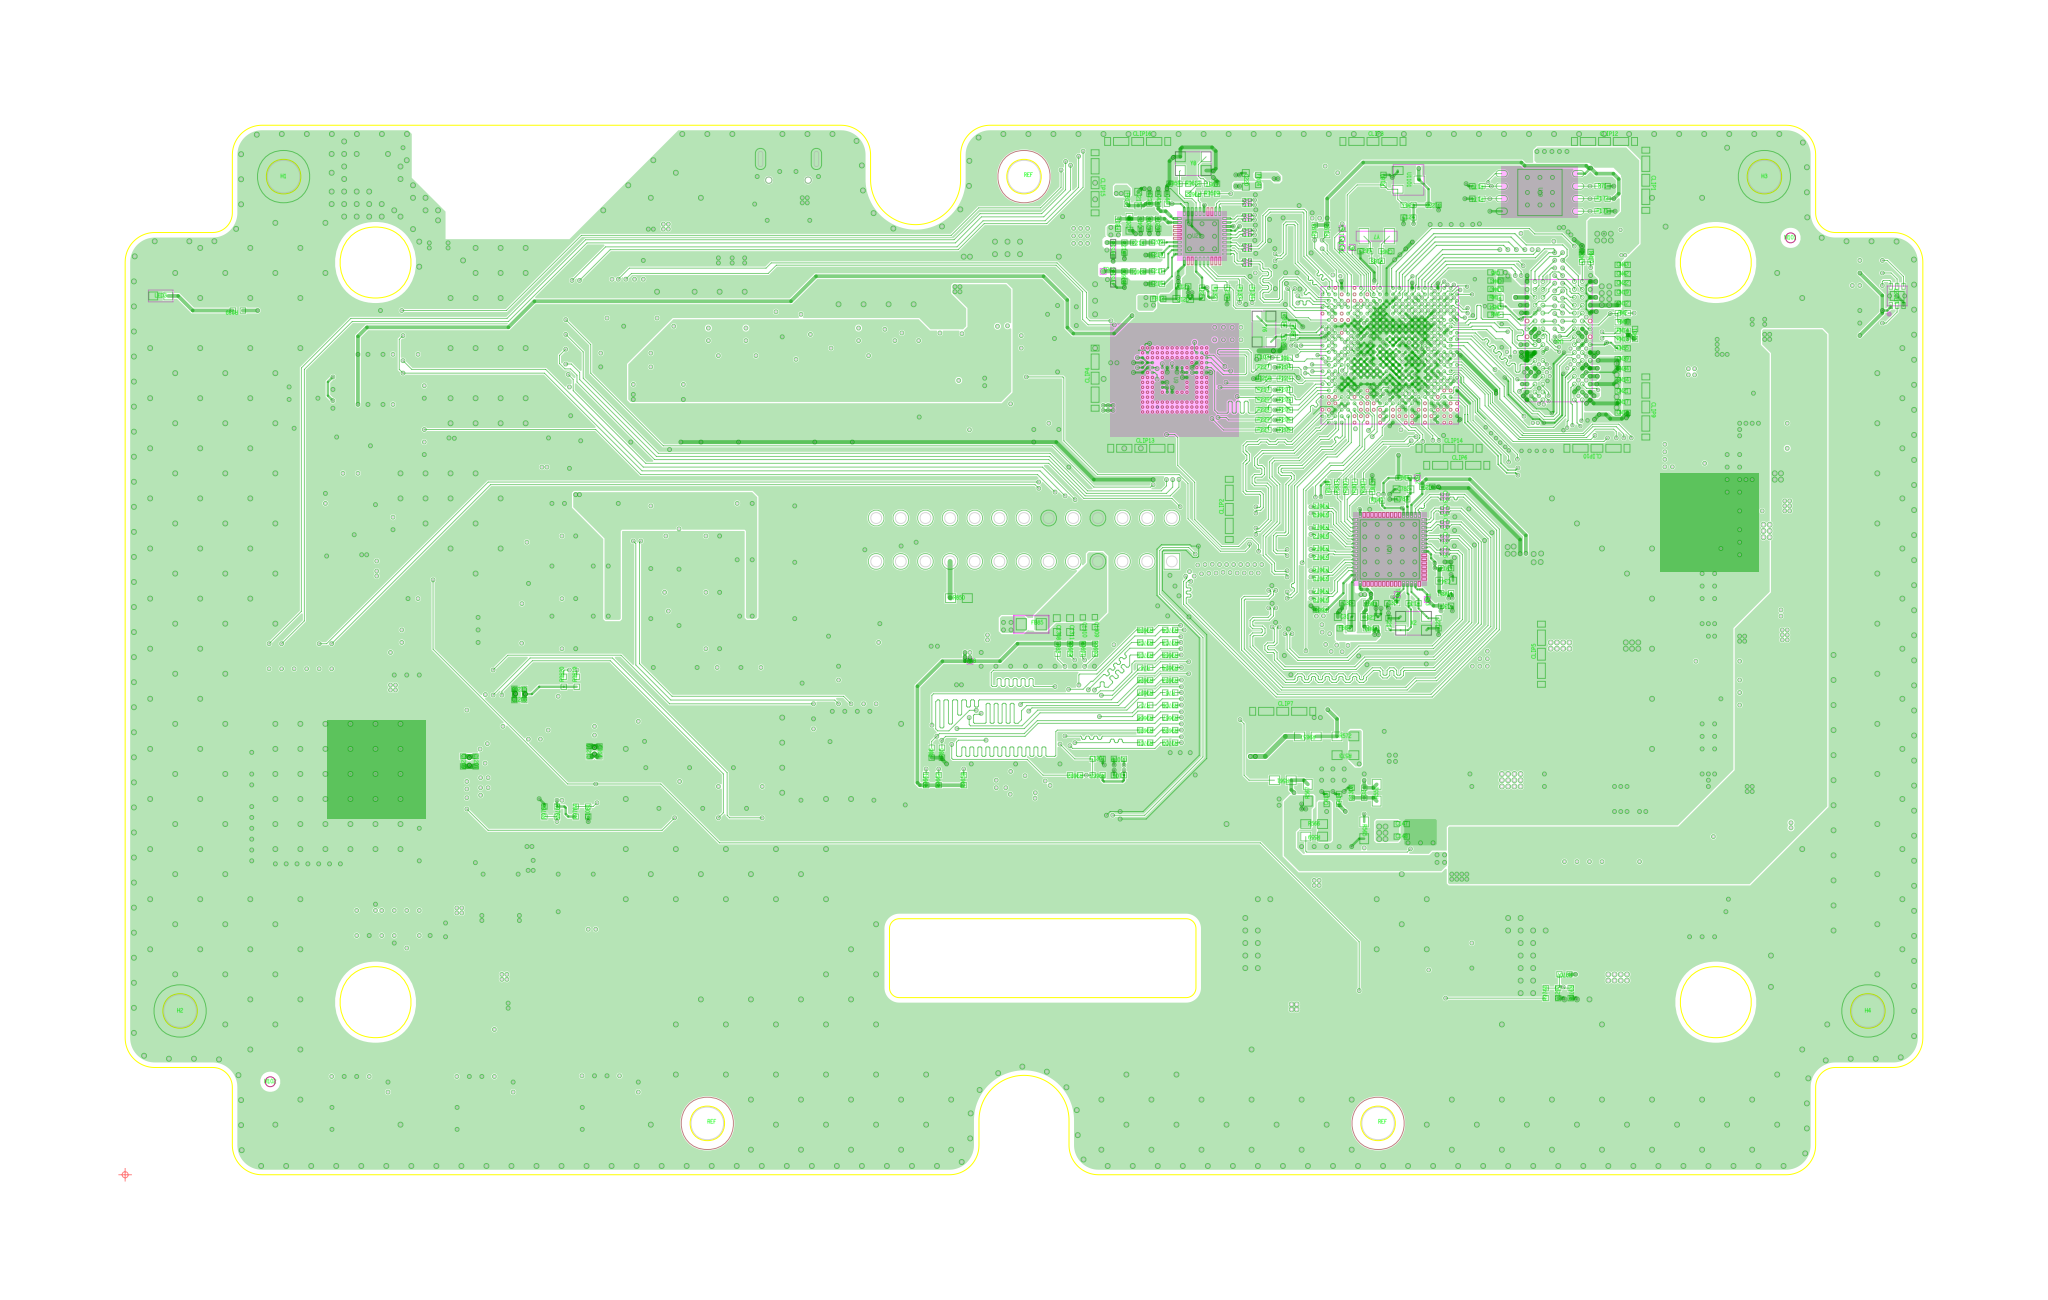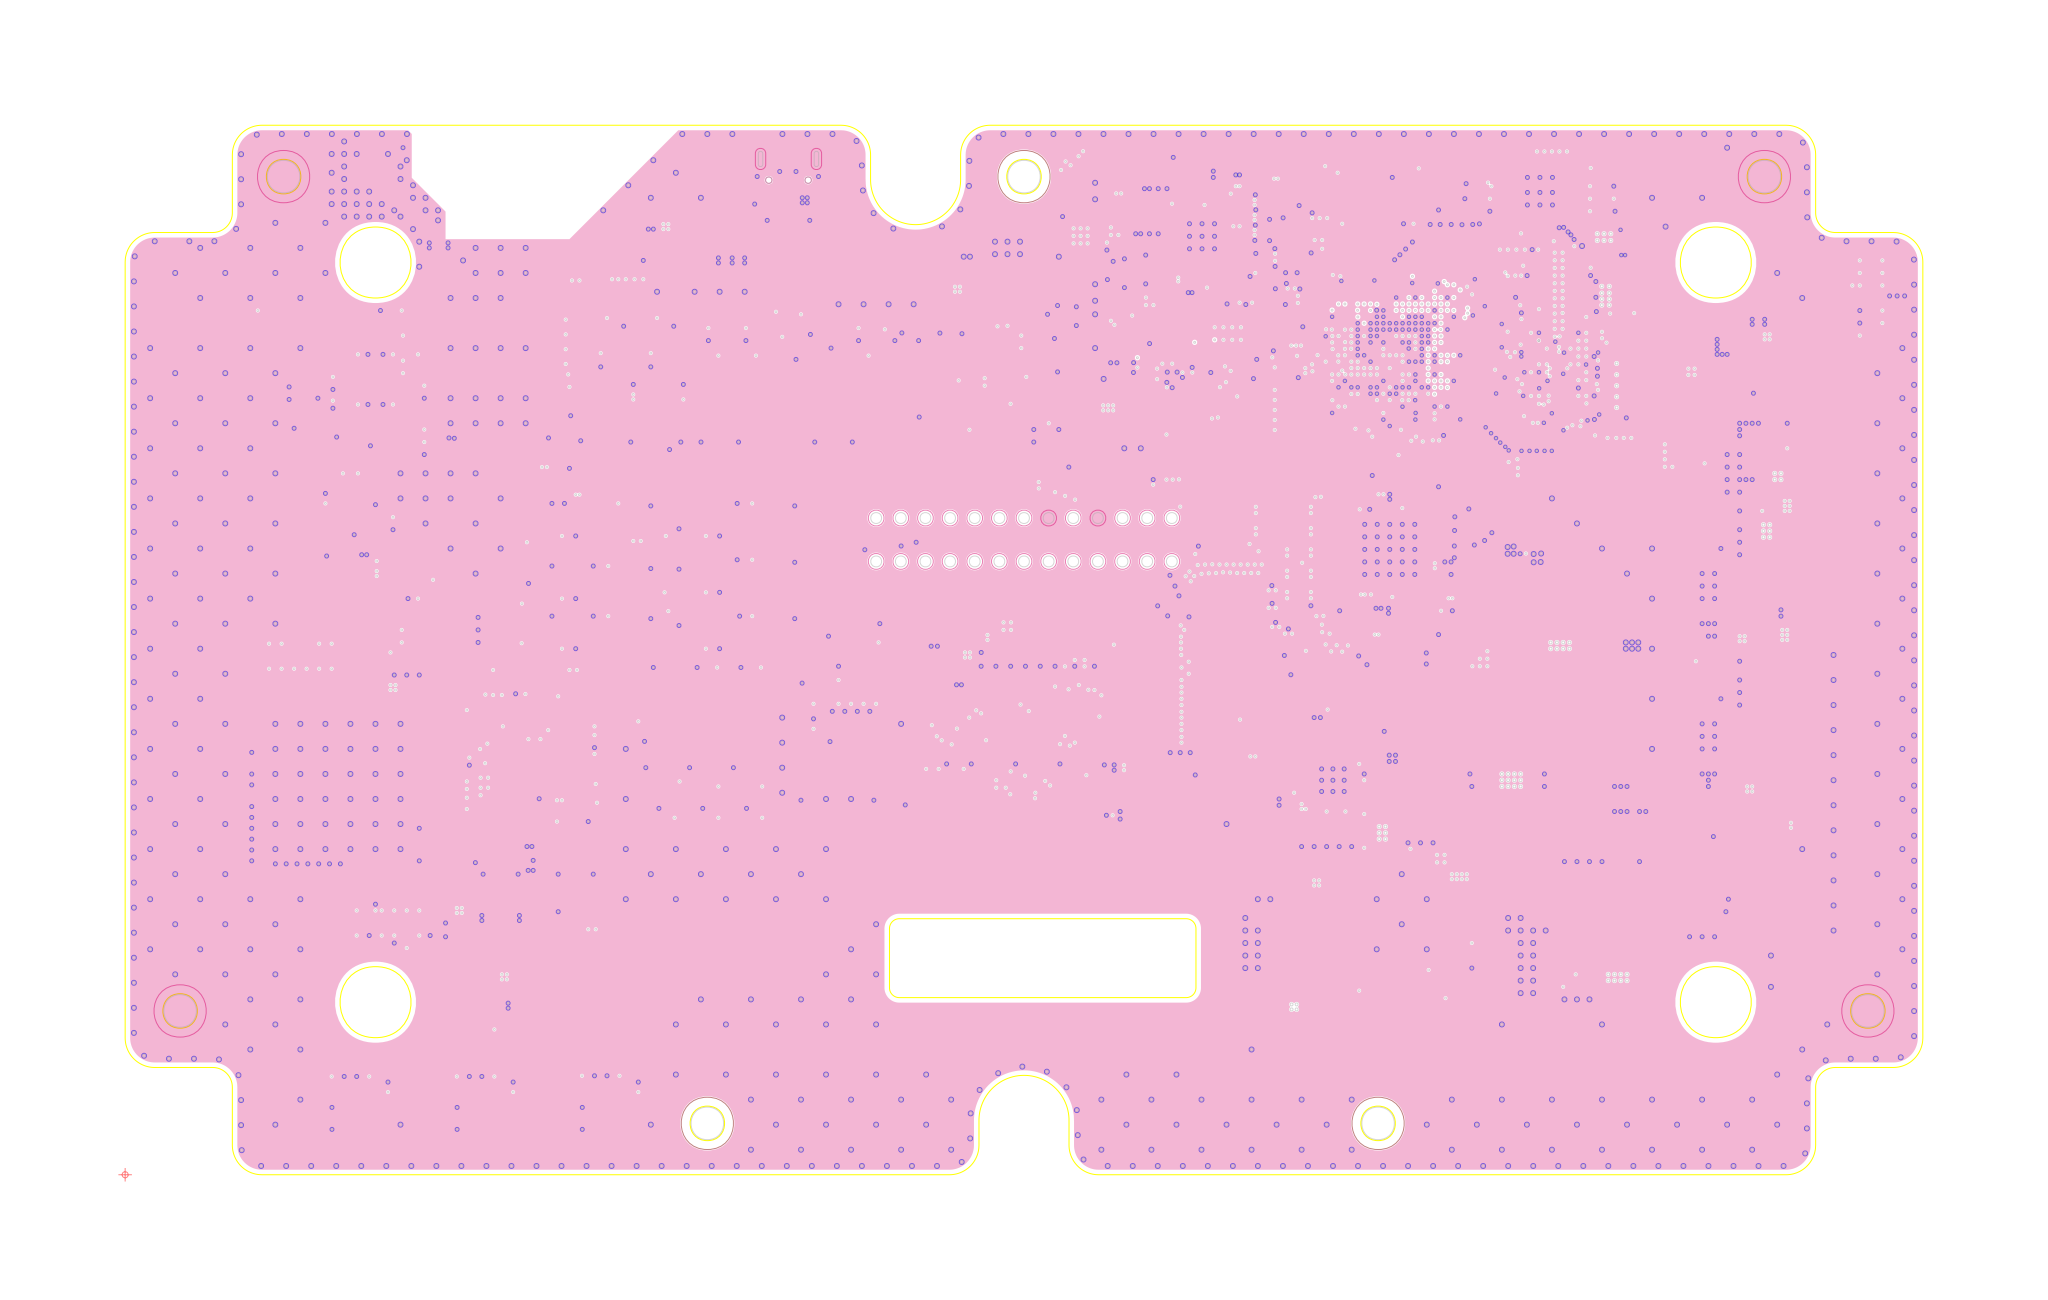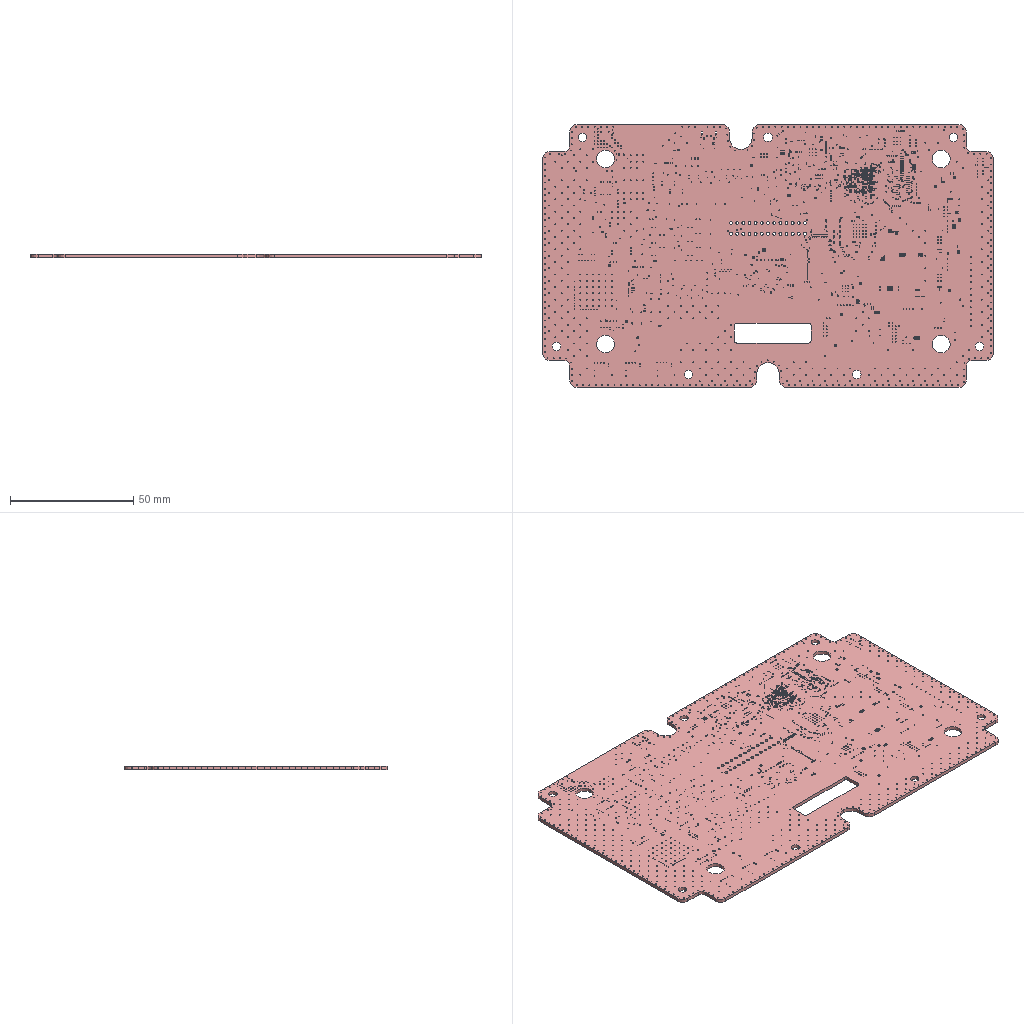Circuit board layout | Cadence Allegro | box 182.4 x 106.4 x 1.5 mm
Layer stack:
# Cadence Allegro layer stack of  (unit mm; from the constraint file cross-section; dielectric type: 0 not recorded (Allegro does not mark core vs prepreg), 3 surface material)
index,name,kind,layer,copper_thickness_mm,dielectric_type,dielectric_thickness_mm,dielectric_material,dielectric_constant
0,Top Surface,other,,,,,,
1,TOP,copper,TOP,0.0356,,,,
2,Dielectric1,dielectric,,,0,0.0737,FR-4,4.5
3,GND02,copper,GND02,0.0305,,,,
4,Dielectric2,dielectric,,,0,0.13,FR-4,4.5
5,ART03,copper,ART03,0.0305,,,,
6,Dielectric3,dielectric,,,0,0.9652,FR-4,4.5
7,PWR04,copper,PWR04,0.0305,,,,
8,Dielectric4,dielectric,,,0,0.13,FR-4,4.5
9,GND05,copper,GND05,0.0305,,,,
10,Dielectric5,dielectric,,,0,0.0737,FR-4,4.5
11,BOTTOM,copper,BOTTOM,0.0356,,,,
12,Bottom Surface,other,,,,,,
# drill layer pairs: low layer,high layer
drill_pair,TOP,BOTTOM
Part placement, first 521 of 963 lines:
REFDES,COMP_VALUE,SYM_NAME,SYM_X,SYM_Y,SYM_ROTATE,SYM_MIRROR
C1,100nF,C0402,6050.00,1300.00,90.000,YES
C3,100nF,C0402,6325.00,1325.00,180.000,YES
C12,1uF,C0402,6250.00,1600.00,180.000,YES
C19,10uF,C0805,6400.00,1550.00,0.000,YES
C20,100nF,C0402,6400.00,1600.00,0.000,YES
C21,15pF,C0402,5047.10,2201.41,270.000,NO
C22,15pF,C0402,5247.10,2201.41,90.000,NO
C23,22uF,C0805,6575.00,2200.00,270.000,YES
C24,100nF,C0402,6500.00,1975.00,0.000,YES
C25,22uF,C0603,6500.00,1875.00,0.000,YES
C28,10uF,C0603,4977.10,2226.41,180.000,NO
C29,100nF,C0402,5202.10,2746.41,180.000,NO
C30,100nF,C0402,5277.10,2271.41,180.000,NO
C31,10uF,C0603,4872.10,2226.41,0.000,NO
C32,100nF,C0402,4882.10,2281.41,0.000,NO
C33,100nF,C0402,5062.10,2281.41,0.000,NO
C34,10uF,C0603,5277.10,2371.41,180.000,NO
C35,100nF,C0402,5077.10,2631.41,270.000,YES
C42,1nF,C0402,4057.10,3796.41,90.000,NO
C43,1nF,C0402,4127.10,3896.41,270.000,NO
C44,1nF,C0402,4162.10,3896.41,270.000,NO
C45,1nF,C0402,4287.10,3856.41,270.000,YES
C66,100nF,C0402,5128.87,3015.50,90.000,YES
C79,0.1uF/16V,C0402,1025.00,350.00,270.000,YES
C102,33pF_NC,C0402,4545.67,3263.06,0.000,NO
C106,100nF,C0402,3970.00,1595.00,180.000,NO
C107,10uF,C0805,3275.00,2150.00,0.000,YES
C122,1uF,C0402,675.00,3075.00,180.000,YES
C123,0.1uF,C0402,675.00,3125.00,180.000,YES
C124,0.1uF,C0402,5127.10,3821.41,0.000,NO
C146,10uF/50V,C1206,5125.00,1375.00,0.000,YES
C147,100nF/50VDC,C0402,5100.00,1400.00,0.000,NO
C148,100nF/50VDC,C0402,5100.00,1350.00,0.000,NO
C201,0.1uF,C0402,6475.00,3375.00,90.000,YES
C202,10uF,C0603,6415.00,3220.00,90.000,YES
C203,0.1uF,C0402,6365.00,3220.00,90.000,YES
C204,10uF/10V,C0603,6525.00,3375.00,90.000,YES
C205,NC/0.1uF,C0402,6330.00,3420.00,0.000,YES
C206,22uF,C0603,4012.10,3796.41,90.000,NO
C207,0.1uF,C0402,4127.10,3796.41,90.000,NO
C208,0.1uF,C0402,4092.10,3796.41,90.000,NO
C209,0.1uF/25V,C0402,4122.10,3721.41,0.000,NO
C210,0.1uF,C0402,4122.10,3671.41,0.000,NO
C211,0.1uF/NC,C0402,4122.10,3606.41,0.000,NO
C212,22uF,C0603,4227.10,3496.41,180.000,NO
C213,0.1uF,C0402,4392.10,3731.41,180.000,YES
C214,0.1uF,C0402,4392.10,3766.41,180.000,YES
C215,0.1uF,C0402,4227.10,3546.41,180.000,NO
C216,0.1uF/NC,C0402,4122.10,3556.41,0.000,NO
C217,22uF,C0603,4047.10,3896.41,270.000,NO
C218,0.1uF,C0402,4092.10,3896.41,270.000,NO
C219,10nF,C0402,4402.10,3521.41,270.000,NO
C220,22uF,C0603,4477.10,3971.41,270.000,NO
C221,0.1uF,C0402,4302.10,3521.41,90.000,NO
C222,0.1uF,C0402,4392.10,3816.41,180.000,YES
C223,0.1uF,C0402,4337.10,3856.41,270.000,YES
C298,22uF,C0603,6500.00,1925.00,0.000,YES
C299,18pF,C0402,4954.88,3686.84,0.000,NO
C300,100nF,C0402,5196.67,3093.06,0.000,YES
C301,10uF,C0603,4887.67,3043.06,0.000,YES
C302,100nF,C0402,4971.36,3324.41,180.000,YES
C303,100nF,C0402,5183.39,3238.14,270.000,YES
C304,100nF,C0402,5177.62,3179.87,0.000,YES
C305,100nF,C0402,5323.87,3238.34,180.000,YES
C306,470nF,C0402,5177.62,3143.76,0.000,YES
C307,10uF,C0603,4979.92,3425.40,0.000,YES
C309,100nF,C0402,4970.01,3370.50,180.000,YES
C310,4.7uF,C0402,5064.89,3015.50,270.000,YES
C311,100nF,C0402,5254.19,3017.82,90.000,YES
C312,4.7uF,C0402,5324.01,3201.18,180.000,YES
C313,100nF,C0402,5477.10,2896.41,0.000,YES
C314,18pF,C0402,4629.76,3411.03,270.000,NO
C315,18pF,C0402,4629.76,3326.03,90.000,NO
C316,100nF,C0402,5026.51,3149.86,90.000,YES
C317,100nF_NI,C0402,5126.96,3218.74,0.000,YES
C318,100nF,C0402,5058.50,3297.00,180.000,YES
C319,10uF,C0603,5072.53,3145.90,270.000,YES
C320,100nF,C0402,4970.01,3283.95,0.000,YES
C327,100nF,C0402,5056.26,3248.18,0.000,YES
C328,100nF,C0402,5119.26,3161.03,90.000,YES
C329,10uF,C0603,5197.67,3025.06,90.000,YES
C330,100nF,C0402,5046.93,3212.39,0.000,YES
C345,10uF,C0603,6400.00,2150.00,180.000,YES
C346,100nF,C0402,6400.00,2200.00,180.000,YES
C347,22uF,C0603,6500.00,2475.00,180.000,YES
C348,22uF,C0603,6500.00,2525.00,180.000,YES
C349,100nF,C0402,6500.00,2575.00,180.000,YES
C350,22pF/50V_NC,C0402,6225.00,2500.00,180.000,YES
C351,1uF,C0402,6250.00,2200.00,0.000,YES
C356,10uF,C0603,4986.89,3159.30,270.000,YES
C357,100nF,C0402,4908.74,3169.05,90.000,YES
C358,100nF,C0402,4908.74,3253.60,270.000,YES
C359,100nF,C0402,4945.38,3169.05,90.000,YES
C360,100nF,C0402,4970.01,3248.19,180.000,YES
C361,100nF,C0402,4947.67,3090.06,180.000,YES
C362,100nF,C0402,4977.67,3054.06,0.000,YES
C363,2.2uF,C0402,5127.10,3871.41,180.000,NO
C364,18pF,C0402,5038.48,3686.84,180.000,NO
C382,100nF,C0402,4872.67,3426.06,0.000,YES
C383,100nF,C0402,5057.67,3072.06,180.000,YES
C384,10uF,C0603,5287.67,3093.06,180.000,YES
C385,100nF,C0402,4872.67,3118.06,270.000,YES
C401,100nF,C0402,4352.67,3423.06,270.000,YES
C402,100nF,C0402,4387.67,3423.06,270.000,YES
C403,100nF,C0402,4422.67,3423.06,270.000,YES
C404,100nF,C0402,4457.67,3423.06,270.000,YES
C405,100nF,C0402,4457.67,3293.06,90.000,YES
C406,100nF,C0402,4422.67,3293.06,90.000,YES
C407,100nF,C0402,4352.67,3293.06,90.000,YES
C408,100nF,C0402,4387.67,3293.06,90.000,YES
C410,470nF/25VDC,C0402,4565.00,1475.00,180.000,YES
C411,1nF_NC,C0402,4650.00,1475.00,0.000,YES
C412,100nF/50VDC,C0402,4625.00,1525.00,0.000,YES
C413,100nF/50VDC,C0402,4800.00,1500.00,90.000,NO
C414,100nF/50VDC,C0402,4850.00,1500.00,90.000,NO
C565,10uF,C0603,4177.67,3068.06,0.000,YES
C566,100nF,C0402,4242.67,3248.06,0.000,YES
C567,100nF,C0402,4177.67,3113.06,0.000,YES
C570,10uF,C0603,3972.67,3273.06,180.000,YES
C572,100nF,C0402,4247.67,3163.06,180.000,YES
C573,100nF,C0402,3977.67,3223.06,180.000,YES
C781,100nF,C0402,4982.10,2746.41,270.000,NO
C782,10uF,C0603,5107.10,2736.41,0.000,NO
C783,100nF,C0402,5102.10,2696.41,0.000,NO
C784,10uF,C0603,4952.10,2621.41,0.000,YES
C841,22uF_0805_10V,C0805,5700.00,1075.00,90.000,YES
C842,22uF_0805_10V,C0805,5625.00,1075.00,90.000,YES
C843,0.1uF/25V,C0402,5525.00,1075.00,270.000,YES
C883,100nF,C0402,4952.10,2676.41,0.000,YES
C897,100nF,C0402,4977.10,2281.41,180.000,NO
C913,100nF,C0402,5277.10,2421.41,180.000,NO
C914,100nF,C0402,1895.00,1690.00,270.000,NO
C915,100nF,C0402,1650.00,1195.00,180.000,YES
C916,100nF,C0402,1650.00,1275.00,180.000,YES
C917,100nF,C0402,1650.00,1235.00,180.000,YES
C919,10uF,C0603,925.00,2450.00,0.000,YES
C920,100nF,C0402,825.00,2450.00,180.000,YES
C921,100nF,C0402,825.00,2700.00,90.000,YES
C944,0.1uF_6.3V,C0402,1800.00,2950.00,270.000,YES
C945,10uF/10V,C0603,1800.00,2850.00,270.000,YES
C946,1uF/25VDC,C0402,5625.00,1600.00,180.000,YES
C947,10pF_50V,C0402,1152.03,3819.69,45.000,YES
C948,10pF_50V,C0402,1067.18,3904.54,45.000,YES
C949,0.1uF_6.3V,C0402,1800.00,3050.00,270.000,YES
C955,22pF,C0402,4782.67,3433.06,90.000,YES
C956,18pF,C0402,4192.10,3956.41,0.000,NO
C957,18pF,C0402,4342.10,3956.41,180.000,NO
C987,100nF/50VDC,C0402,3445.00,2855.00,180.000,YES
C988,100nF/50VDC,C0402,4225.00,2847.00,180.000,YES
C990,100uF/50V,EC-6_6X6_6-P4_6-H7_7,6200.00,1000.00,180.000,YES
C995,22uF,C0805,3675.00,3600.00,270.000,YES
C996,100nF,C0402,3730.00,3600.00,270.000,YES
C997,22pF/50V_NC,C0402,3700.00,3775.00,0.000,YES
C1001,22uF/10V,C0805,6375.00,2925.00,180.000,YES
C1002,100nF,C0402,6350.00,2875.00,180.000,YES
C1006,10uF,C0805,4600.00,1050.00,0.000,YES
C1007,100nF,C0402,4600.00,1125.00,0.000,YES
C1008,22pF/50V,C0402,4450.00,1100.00,90.000,YES
C1014,22uF/10V,C0805,6375.00,3000.00,180.000,YES
C1015,1uF,C0402,6350.00,2840.00,180.000,YES
C1036,22pF/10V,C0402,6600.00,2900.00,0.000,YES
C1053,2.2uF/50VDC,C0603,5425.00,1600.00,0.000,YES
C1054,100nF/50VDC,C0402,5425.00,1550.00,0.000,YES
C1055,1uF/25VDC,C0402,5625.00,1550.00,180.000,YES
C1056,220uF/50V,AP-SMD_BD6_3-L6_6-W6_6-LS7_21,5875.00,1500.00,180.000,YES
C1061,1uF/25VDC,C0402,4136.00,2848.00,0.000,YES
C1062,100nF/50VDC,C0402,3390.00,3165.00,0.000,YES
C1063,100nF/50VDC,C0402,3445.00,2890.00,180.000,YES
C1064,1uF/25VDC,C0402,3445.00,2925.00,180.000,YES
C1068,1uF,C0402,6525.00,3100.00,270.000,YES
C1069,100nF,C0402,6540.00,2790.00,0.000,YES
C1070,10uF,C0805,6540.00,2740.00,0.000,YES
C1071,0.1uF/25V,C0402,5575.00,1075.00,270.000,YES
C1072,100nF/50VDC,C0402,2125.00,3750.00,180.000,YES
C1073,10uF/10V,C0603,2400.00,3675.00,270.000,YES
C1074,100nF/50VDC,C0402,2450.00,3675.00,270.000,YES
C1075,0.1uF/16V,C0402,2025.00,350.00,270.000,YES
C1076,10uF,C0805,3275.00,2075.00,0.000,YES
C1077,100nF,C0402,3400.00,2110.00,180.000,YES
C1079,100nF,C0402,3970.00,1660.00,180.000,NO
C1081,100nF,C0402,1850.00,1450.00,90.000,NO
C1082,0.1uF/16V,C0402,1525.00,350.00,270.000,YES
C1085,100nF,C0402,3650.00,3000.00,180.000,YES
C1087,100nF/50VDC,C0402,1150.00,2275.00,180.000,YES
C1200,100nF,C0402,1150.00,3100.00,180.000,YES
C1201,100nF,C0402,1150.00,2875.00,180.000,YES
C1202,100nF,C0402,1050.00,3250.00,0.000,YES
C1203,100nF,C0402,950.00,3250.00,180.000,YES
C1204,100nF,C0402,1050.00,3050.00,0.000,YES
C1205,100nF,C0402,950.00,3050.00,180.000,YES
C1206,10nF,C0402,1575.00,1895.00,0.000,NO
C1207,10nF_X7R,C0402,1400.00,1650.00,270.000,NO
C1208,1uF/16V_X7R,C0402,1575.00,1940.00,180.000,NO
C1209,1uF/16V_X7R,C0402,1350.00,1650.00,270.000,NO
C1210,4.7F/16V_X7R,C0402,1855.00,1690.00,90.000,NO
C1211,12PF/50VDC_NC,C0402,1750.00,1225.00,180.000,YES
C1212,12PF/50VDC_NC,C0402,1850.00,1225.00,0.000,YES
C1213,12PF/50VDC,C0402,1450.00,1225.00,180.000,YES
C1214,12PF/50VDC,C0402,1550.00,1225.00,0.000,YES
C1215,10uF_10V,C0603,1450.00,1000.00,90.000,YES
C1230,10uF_10V,C0603,1300.00,975.00,180.000,YES
C1231,4.7uF_10V,C0603,1350.00,1225.00,0.000,YES
C1235,0.1uF,C0402,5227.10,3871.41,180.000,NO
C1237,68nF_X7R/50VDC,C0402,975.00,2700.00,270.000,YES
C1238,5.6pF_50V_NC,C0402,975.00,1000.00,90.000,YES
C1239,2.2uF/50VDC,C0603,5900.00,1300.00,90.000,YES
C1240,100nF/50VDC,C0402,5850.00,1300.00,90.000,YES
C1241,100nF/50VDC,C0402,5750.00,1300.00,90.000,YES
C1242,100nF/50VDC,C0402,5800.00,1300.00,90.000,YES
C1243,100nF/50VDC,C0402,3700.00,3225.00,90.000,YES
C1248,100nF/50VDC,C0402,1100.00,1975.00,270.000,YES
C1249,100nF/50VDC,C0402,1150.00,1975.00,270.000,YES
C1250,100nF/50VDC,C0402,1200.00,1975.00,270.000,YES
C1251,100nF/50VDC,C0402,1550.00,1000.00,270.000,YES
C1252,100nF/50VDC,C0402,1580.00,760.00,180.000,YES
C1253,100nF/50VDC,C0402,1400.00,1000.00,270.000,YES
C1254,100nF/50VDC,C0402,1300.00,1025.00,0.000,YES
C1255,10uF_10V,C0603,1600.00,1000.00,90.000,YES
C1256,100nF,C0402,4212.67,3333.06,90.000,YES
C1257,2.2uF,C0402,4247.67,3333.06,90.000,YES
C1258,5.6pF_50V_NC,C0402,4547.67,3178.06,0.000,NO
C1259,10uF_10V,C0603,3325.00,3600.00,90.000,YES
C1260,100nF/50VDC,C0402,3375.00,3600.00,90.000,YES
C1261,10uF_10V,C0603,6450.00,1050.00,180.000,YES
C1262,100nF/50VDC,C0402,6450.00,1100.00,180.000,YES
C1263,10uF_10V,C0603,5875.00,750.00,270.000,YES
C1264,1uF/50V,C0603,5775.00,750.00,270.000,YES
C1265,0.1uF/50V,C0603,5825.00,750.00,270.000,YES
C1266,100nF_25V,C0402,5775.00,875.00,270.000,YES
C1267,68pF_50V,C0402,5400.00,750.00,180.000,YES
C1268,10uF/50V,C1206,4750.00,1925.00,270.000,YES
C1269,100nF/50VDC,C0402,4675.00,1950.00,90.000,YES
C1270,100nF/50VDC,C0402,4625.00,1950.00,90.000,YES
C1271,100nF/50VDC,C0402,4575.00,1950.00,90.000,YES
C1273,10uF,C0805,4575.00,675.00,0.000,YES
C1274,100nF,C0402,4575.00,725.00,0.000,YES
C1275,100nF/50VDC,C0402,3375.00,3725.00,90.000,YES
C1276,100nF,C0402,4425.00,725.00,180.000,YES
C1277,10uF_10V,C0603,6425.00,1345.00,180.000,YES
C1278,100nF/50VDC,C0402,6425.00,1395.00,180.000,YES
C1280,100nF/50VDC,C0402,2700.00,3275.00,0.000,YES
C1283,100nF/50VDC,C0402,2350.00,3350.00,0.000,YES
C1284,100nF/50VDC,C0402,2500.00,3350.00,0.000,YES
C1285,100nF-50V/NC,C0402,2950.00,3350.00,0.000,YES
C1286,100nF/50VDC,C0402,2425.00,2475.00,180.000,YES
C1287,100nF/50VDC,C0402,2250.00,3175.00,90.000,YES
C1289,100nF/50VDC,C0402,2050.00,1750.00,90.000,YES
C1290,100nF/50VDC,C0402,1850.00,2250.00,180.000,YES
C1291,100nF/50VDC,C0402,2425.00,2250.00,180.000,YES
C1292,100nF/50VDC,C0402,1850.00,2450.00,180.000,YES
C1293,100nF/50VDC,C0402,1775.00,2675.00,270.000,YES
C1294,100nF/50VDC,C0402,2275.00,1650.00,0.000,YES
C1295,100nF/50VDC,C0402,2450.00,1650.00,0.000,YES
C1296,100nF/50VDC,C0402,2850.00,2075.00,90.000,YES
C1297,100nF,C0402,5725.00,725.00,90.000,NO
C1299,100nF/50VDC_NC,C0402,4980.00,1635.00,90.000,YES
C1300,100nF/50VDC,C0402,6975.00,3450.00,0.000,YES
C1301,100nF/50VDC,C0402,3885.00,1660.00,0.000,NO
C1302,100nF/50VDC,C0402,2775.00,1800.00,270.000,YES
C1303,1uF/25V,C0402,4900.00,1525.00,90.000,NO
C1304,22pF/50V_NC,C0402,6225.00,1900.00,180.000,YES
C1305,100nF/50VDC,C0402,2050.00,3175.00,90.000,YES
C1306,100nF/50VDC,C0402,2425.00,2700.00,180.000,YES
C1307,100nF/50VDC,C0402,3095.00,3310.00,0.000,YES
C1308,2.2uF/50VDC,C0603,3722.00,2194.36,270.000,NO
C1309,1uF/25VDC,C0402,3874.00,2206.00,270.000,NO
C1310,100nF/50VDC,C0402,3826.00,2205.00,270.000,NO
C1311,10uF,C0603,3775.00,2194.36,270.000,NO
CL22,90OHM_400mA,ESD4_0_9X0_7H0,5272.10,2541.41,270.000,NO
CL23,90OHM_400mA,ESD4_0_9X0_7H0,5272.10,2706.41,270.000,NO
CL24,90OHM_400mA,ESD4_0_9X0_7H0,5272.10,2651.41,270.000,NO
CL25,90OHM_400mA,ESD4_0_9X0_7H0,5272.10,2596.41,270.000,NO
CL26,90OHM_400mA,ESD4_0_9X0_7H0,5272.10,2486.41,270.000,NO
CLIP1,DCL-PBJ001,PBJ-01,6075.00,3970.00,270.000,NO
CLIP2,DCL-PBJ001,PBJ-01,4411.00,2656.05,90.000,NO
CLIP3,DCL-PBJ001,PBJ-01,4985.00,4125.00,0.000,NO
CLIP4,DCL-PBJ001,PBJ-01,3875.00,3180.00,90.000,NO
CLIP5,DCL-PBJ001,PBJ-01,5658.00,2077.91,90.000,NO
CLIP6,DCL-PBJ001,PBJ-01,5319.68,2832.00,0.000,NO
CLIP7,DCL-PBJ001,PBJ-01,4624.49,1850.00,0.000,NO
CLIP8,DCL-PBJ001,PBJ-01,4513.00,3228.00,90.000,YES
CLIP9,DCL-PBJ001,PBJ-01,6075.00,3065.00,270.000,NO
CLIP10,DCL-PBJ001,PBJ-01,5879.88,2900.00,180.000,NO
CLIP11,DCL-PBJ001,PBJ-01,6096.00,3644.00,90.000,YES
CLIP12,DCL-PBJ001,PBJ-01,5910.00,4125.00,0.000,NO
CLIP13,DCL-PBJ001,PBJ-01,4057.49,2900.00,0.000,NO
CLIP14,DCL-PBJ001,PBJ-01,5289.11,2900.00,0.000,NO
CLIP15,DCL-PBJ001,PBJ-01,3875.00,3960.00,270.000,NO
CLIP16,DCL-PBJ001,PBJ-01,4045.00,4125.00,0.000,NO
CLIP18,DCL-PBJ001,PBJ-01,5803.81,2797.00,0.000,YES
CLIP19,DCL-PBJ001,PBJ-01,4986.28,2797.00,0.000,YES
CLIP20,DCL-PBJ001,PBJ-01,6125.00,2551.86,90.000,YES
CLIP21,DCL-PBJ001,PBJ-01,6700.00,3052.14,90.000,YES
CLIP22,DCL-PBJ001,PBJ-01,4334.00,885.00,90.000,YES
CLIP23,DCL-PBJ001,PBJ-01,4588.07,600.00,0.000,YES
CLIP24,DCL-PBJ001,PBJ-01,4475.00,1451.68,90.000,YES
CLIP25,DCL-PBJ001,PBJ-01,4850.00,886.18,90.000,YES
CLIP26,DCL-PBJ001,PBJ-01,5325.00,1559.86,90.000,YES
CLIP27,DCL-PBJ001,PBJ-01,6125.00,1961.28,90.000,YES
CLIP28,DCL-PBJ001,PBJ-01,6125.00,2441.25,90.000,YES
CLIP29,DCL-PBJ001,PBJ-01,6700.00,1957.78,90.000,YES
CLIP30,DCL-PBJ001,PBJ-01,4878.60,2050.00,0.000,YES
CLIP31,DCL-PBJ001,PBJ-01,5827.12,3990.00,0.000,YES
CLIP32,DCL-PBJ001,PBJ-01,5104.54,3990.00,0.000,YES
CM1,10uF,C0603,5057.49,3373.89,270.000,YES
CM2,100nF,C0402,5116.94,3370.43,270.000,YES
CM3,100nF,C0402,5150.64,3370.43,270.000,YES
CM4,100nF,C0402,5150.64,3289.73,90.000,YES
CM5,4.7uF,C0402,5474.10,3602.41,180.000,NO
CM6,100nF,C0402,5116.94,3289.73,270.000,YES
CM11,10uF,C0603,5453.00,3597.27,0.000,YES
CM12,100nF,C0402,5982.74,3477.24,0.000,NO
CM13,100nF,C0402,5982.74,3172.12,180.000,YES
CM14,100nF,C0402,5982.74,3172.12,0.000,NO
CM15,100nF,C0402,5982.74,3216.41,180.000,YES
CM16,100nF,C0402,5982.74,3127.83,180.000,YES
CM17,100nF,C0402,5982.74,3083.54,0.000,NO
CM18,100nF,C0402,5982.74,3041.53,0.000,NO
CM19,100nF,C0402,5982.74,3521.53,0.000,NO
CM20,100nF,C0402,5982.74,3083.54,180.000,YES
CM21,100nF,C0402,5982.74,3127.83,0.000,NO
CM22,100nF,C0402,5982.74,3558.98,0.000,NO
CM23,100nF,C0402,5982.74,3477.24,180.000,YES
CM24,100nF,C0402,5982.34,3260.84,180.000,YES
CM25,100nF,C0402,5476.27,3540.88,0.000,YES
CM26,100nF,C0402,5982.74,3298.15,180.000,YES
CM31,10uF,C0603,5972.90,3605.19,270.000,YES
CM32,100nF,C0402,5982.74,3521.53,180.000,YES
CM33,100nF,C0402,5476.27,3502.53,0.000,YES
CM34,100nF,C0402,5982.74,3216.41,0.000,NO
CM35,100nF,C0402,5497.07,3437.53,90.000,YES
CM36,100nF,C0402,5497.07,3348.80,270.000,YES
CM37,100nF,C0402,5497.17,3093.18,270.000,YES
CM38,100nF,C0402,5982.74,3041.53,180.000,YES
CM39,100nF,C0402,5982.74,3255.78,0.000,NO
CM40,100nF,C0402,5474.47,3536.37,180.000,NO
CM41,100nF,C0402,5474.47,3569.72,180.000,NO
CM42,100nF,C0402,5982.74,3595.89,0.000,NO
CM43,100nF,C0402,5982.74,3632.36,0.000,NO
CM44,100nF,C0402,5497.07,3263.97,270.000,YES
CM45,100nF,C0402,5497.07,3177.52,270.000,YES
CM51,10nF,C0402,6032.10,3356.41,90.000,NO
CM52,100nF,C0402,5820.10,3664.01,90.000,NO
CM53,100nF,C0402,5726.81,3741.23,270.000,YES
CM54,1nF,C0402,5474.47,3466.41,180.000,NO
CM55,100nF,C0402,5982.74,3299.15,0.000,NO
CON2,FPC_6PINB_Up_Type,FPC_6PINB,2875.00,1675.00,0.000,YES
CON5,FPC50PM-0.5mm-B,ZIF50-S0_5-29_2X5_35X2G,3665.70,1675.89,0.000,YES
CON26,FPC40PM-0.5mm-B,CON40-P0_5-H2,3665.70,1890.89,0.000,YES
D2,D2_NC,R0402,4950.00,1525.00,90.000,NO
D42,JEB05LCDF,DFN1006,2825.00,1800.00,270.000,YES
D43,JEB05LCDF,DFN1006,2875.00,1800.00,270.000,YES
D44,JEB05LCDF,DFN1006,2925.00,1800.00,270.000,YES
D45,JEB05LCDF,DFN1006,2975.00,1800.00,270.000,YES
D49,SS34,SMB,4875.00,1875.00,270.000,YES
D50,SS34,SMB,5165.00,1735.00,180.000,YES
D67,PESD1IVN27-A,SOD_323,2125.00,2625.00,90.000,YES
D68,S2M,DO-214AA,1950.00,2600.00,0.000,YES
D72,PESD1IVN27-A,SOD_323,2325.00,2000.00,180.000,YES
D73,S2M,DO-214AA,2325.00,1825.00,270.000,YES
D74,PESD1IVN27-A,SOD_323,2500.00,2000.00,180.000,YES
D75,S2M,DO-214AA,2500.00,1825.00,270.000,YES
D76,PESD1IVN27-A,SOD_323,2980.00,2175.00,90.000,YES
D77,S2M,DO-214AA,3025.00,2025.00,180.000,YES
D78,PESD1IVN27-A,SOD_323,2700.00,2175.00,90.000,YES
D79,S2M,DO-214AA,2525.00,2150.00,0.000,YES
D80,PESD1IVN27-A,SOD_323,2125.00,2175.00,90.000,YES
D81,S2M,DO-214AA,1950.00,2150.00,0.000,YES
D82,PESD1IVN27-A,SOD_323,2150.00,2000.00,180.000,YES
D83,S2M,DO-214AA,2150.00,1825.00,90.000,YES
D89,PESD1IVN27-A,SOD_323,2800.00,2900.00,180.000,YES
D90,S2M,DO-214AA,2725.00,3175.00,0.000,YES
D91,S2M,DO-214AA,2725.00,3025.00,0.000,YES
D92,PESD1IVN27-A,SOD_323,2125.00,2375.00,90.000,YES
D93,S2M,DO-214AA,1950.00,2350.00,0.000,YES
D95,PESD1IVN27-A,SOD_323,2350.00,2900.00,180.000,YES
D97,S2M,DO-214AA,2350.00,3075.00,270.000,YES
D98,S2M,DO-214AA,2500.00,3075.00,270.000,YES
D99,PESD1IVN27-A,SOD_323,2500.00,2900.00,180.000,YES
D100,PESD1IVN27-A/NC,SOD_323,2950.00,2900.00,180.000,YES
D101,S2M/NC,DO-214AA,2950.00,3075.00,270.000,YES
D112,LED_RED,LED-0603,1050.00,3400.00,180.000,YES
D113,SS34,SMB,5625.00,1775.00,90.000,YES
D132,SS34,SMB,5800.00,1775.00,90.000,YES
D134,SS34,SMB,5975.00,1775.00,90.000,YES
D135,SS34,SMB,5450.00,1775.00,90.000,YES
D137,SS34,SMB,2400.00,3875.00,270.000,YES
D140,PESD1IVN27-A,SOD_323,2700.00,2400.00,90.000,YES
D141,S2M,DO-214AA,2525.00,2375.00,0.000,YES
D142,S2M,D0214AAH2_42,5275.00,725.00,90.000,YES
D143,PESD1IVN27-A,SOD_323,3775.00,2950.00,180.000,YES
D145,S2M,D0214AAH2_42,5025.00,650.00,180.000,YES
D146,PESD1IVN27-A,SOD_323,2175.00,2900.00,0.000,YES
D147,S2M,DO-214AA,2150.00,3075.00,270.000,YES
D148,S2M,DO-214AA,3700.00,3100.00,180.000,YES
D149,PESD1IVN27-A,SOD_323,2700.00,2625.00,90.000,YES
D150,S2M,DO-214AA,2525.00,2600.00,0.000,YES
D151,PESD1IVN27-A,SOD_323,1975.00,2900.00,0.000,YES
D152,S2M,DO-214AA,1950.00,3075.00,270.000,YES
D153,PESD1IVN27-A,SOD_323,3125.00,3055.00,0.000,YES
D154,S2M,DO-214AA,3165.00,3169.50,180.000,YES
D155,S2M,DO-214AA,3180.00,2914.50,180.000,YES
FB6,FB120R,L0402,5096.88,3015.50,270.000,YES
FB11,120R@100MHz,R0402,3967.10,3796.41,90.000,NO
FB12,120R@100MHz,R0402,4127.10,3496.41,0.000,NO
FB13,120R@100MHz,R0402,4002.10,3896.41,270.000,NO
FB14,1K@100MHz,R0402,4527.10,3971.41,270.000,NO
FB23,1K@100MHz,R0603,3987.10,3136.41,270.000,YES
FB64,HCB1005KF-221T15,R0402,4872.10,2181.41,0.000,NO
FB65,HCB1005KF-221T15,R0402,5277.10,2321.41,180.000,NO
FB66,HCB1005KF-221T15,R0402,5107.10,2781.41,0.000,NO
FB79,HCB1005KF-221T15,R0402,4927.10,2556.41,270.000,YES
FB80,HCB1005KF-221T15,R0402,4977.10,2181.41,180.000,NO
FB81,330R@100MHz,R0603,925.00,2400.00,0.000,YES
FB82,120R@100MHz,R0402,1725.00,2825.00,180.000,YES
FB84,330R@100MHz,R0603,1660.00,1110.00,270.000,YES
FB85,600R@100MHz,R0805,3620.00,2197.50,0.000,NO
H1,HOLE,MTH_5_3D3_3,632.96,3984.61,0.000,NO
H2,HOLE,MTH_5_3D3_3,219.57,653.90,0.000,NO
H3,HOLE,MTH_5_3D3_3,6548.85,3984.61,0.000,NO
H4,HOLE,MTH_5_3D3_3,6962.24,653.90,0.000,NO
J1,IPEX1,RF_3X3_1H1_25,964.64,4035.36,225.000,YES
J3,MICRO USB_B,USB5_5X6_9H2_35_L1_6,2650.00,3940.94,180.000,YES
J6,1.25-4P,CON4-P1_25-10X4_2-H3_65,900.00,225.00,180.000,YES
J7,1.25-4P,CON4-P1_25-10X4_2-H3_65,1900.00,225.00,180.000,YES
J8,1.25-4P,CON4-P1_25-10X4_2-H3_65,1400.00,225.00,180.000,YES
L3,1uH,L-2_8X2-P2,6575.00,1775.00,270.000,YES
L4,1uH/2.7A,L-2_8X2-P2,6575.00,2375.00,270.000,YES
L5,FB60R/300mA,L0402,5229.67,2954.06,0.000,YES
L6,WIP252010P-1R0ML,L-2_8X2-P2,6500.00,3235.00,90.000,YES
L12,SDMM0806H-2-900T,ESD4_0_9X0_7H0,4482.10,3641.41,90.000,NO
L13,SDMM0806H-2-900T,ESD4_0_9X0_7H0,4482.10,3701.41,90.000,NO
L14,SDMM0806H-2-900T,ESD4_0_9X0_7H0,4482.10,3761.41,90.000,NO
L19,10uH,IND-5X5,5225.00,1925.00,0.000,YES
L20,600R@100MHz__25%_NC,R0805,5925.00,2000.00,90.000,YES
L21,TMPC0503HV-100MG-D,IND-5X5,5475.00,1425.00,180.000,YES
L22,600R@100MHz__25%_NC,R0805,5825.00,2000.00,90.000,YES
L23,ACM2012/NC,ESD4_0_9X0_7H0,900.00,2700.00,90.000,YES
L24,SDMM0806H-2-900T,ESD4_0_9X0_7H0,4482.10,3881.41,90.000,NO
L25,SDMM0806H-2-900T,ESD4_0_9X0_7H0,4482.10,3821.41,90.000,NO
L28,6.8uH_4.5A,L-6X6-P4_5-H2,5875.00,1075.00,270.000,YES
L29,600R@100MHz__25%,R0805,5475.00,2000.00,90.000,YES
L30,600R@100MHz__25%,R0805,5575.00,2000.00,90.000,YES
L31,1uH,L-2_8X2-P2,4750.00,925.00,270.000,YES
L32,1uH,L-2_8X2-P2,3575.00,3475.00,180.000,YES
L33,1uH,L-2_8X2-P2,6375.00,3100.00,0.000,YES
L35,WCM2012F2SF-900T04,ESD4_0_9X0_7H0,2650.00,3675.00,0.000,YES
LED3,LED_0603,LED-0603,142.08,3508.24,0.000,NO
M101,T_POINT,MARK2,6653.53,3740.15,0.000,NO
M102,T_POINT,MARK2,579.83,371.27,0.000,NO
M103,T_POINT,MARK2,579.83,371.27,0.000,YES
M104,T_POINT,MARK2,6653.53,3740.15,0.000,YES
Q1,2N7002,SOT-23,3505.00,3265.00,180.000,YES
Q5,2N7002,SOT-23,6350.00,2000.00,180.000,YES
Q13,PMV48XPA,SOT-23,3365.00,3065.00,180.000,YES
Q15,L2SA1037AKQLT1G,SOT-23,5352.10,2896.41,270.000,YES
Q17,2N7002,SOT-23,6350.00,2600.00,180.000,YES
Q21,N-MOS_QM3002N3,N_MOS_QM3002N3,5150.00,1525.00,180.000,YES
Q31,PMV48XPA,SOT23-123,1675.00,2650.00,0.000,YES
Q33,MMBT5551,SOT23-123,2300.00,1500.00,90.000,YES
Q34,MMBT5551,SOT23-123,2475.00,1500.00,90.000,YES
Q35,MMBT5551,SOT23-123,2700.00,2000.00,90.000,YES
Q36,MMBT5551,SOT23-123,2250.00,2200.00,0.000,YES
Q37,MMBT5551,SOT23-123,1675.00,2200.00,0.000,YES
Q38,MMBT5551,SOT23-123,2125.00,1500.00,90.000,YES
Q41,MMBT5551,SOT23-123,2775.00,3425.00,0.000,YES
Q42,MMBT5551,SOT23-123,1675.00,2400.00,0.000,YES
Q52,MMBT5551,SOT23-123,2250.00,2425.00,0.000,YES
Q53,MMBT5551,SOT-23,3750.00,3350.00,0.000,YES
Q55,MMBT5551,SOT23-123,2200.00,3350.00,270.000,YES
Q56,PMV48XPA,SOT-23,1605.00,865.00,0.000,YES
Q57,MMBT5551,SOT-23,3355.00,3320.00,270.000,YES
Q61,MMBT5551,SOT23-123,2250.00,2650.00,0.000,YES
Q62,MMBT5551,SOT23-123,2000.00,3350.00,270.000,YES
Q63,2N7002,SOT-23,3500.00,3065.00,180.000,YES
Q64,MMBT5551,SOT23-123,3170.00,3400.00,0.000,YES
R1,NC(0R),R1206,6175.00,1275.00,180.000,YES
R2,NC(0R),R1206,6175.00,1200.00,180.000,YES
R3,1K_1%,R0402,3505.00,3365.00,180.000,YES
R4,1.5K_1%,R0402,3575.00,2875.00,90.000,YES
R5,1K_1%,R0402,3510.00,3165.00,180.000,YES
R6,1.5K_1%,R0402,3510.00,2875.00,90.000,YES
R17,100K,R0402,6250.00,1550.00,180.000,YES
R18,0R,R0603,6600.00,2025.00,270.000,YES
R19,10K/1%,R0402,6225.00,1950.00,0.000,YES
R21,18K/1%,R0402,6325.00,1900.00,0.000,YES
R22,90K/1%,R0402,6225.00,2000.00,0.000,YES
R34,3.3R,R0402,2625.00,3675.00,270.000,YES
R35,3.3R,R0402,2675.00,3675.00,270.000,YES
R42,20K,R0402,4177.67,3333.06,90.000,YES
R51,2.2K,R0402,1150.00,3200.00,180.000,YES
R52,2.2K,R0402,1150.00,3250.00,180.000,YES
R53,33R,R0402,1150.00,2975.00,0.000,YES
R71,NC/4K7,R0402,5902.10,3946.41,0.000,NO
R74,33R,R0402,4075.00,2025.00,180.000,NO
R75,33R,R0402,4075.00,1875.00,180.000,NO
R76,33R,R0402,4175.00,1925.00,180.000,NO
R81,33R,R0402,4632.67,3262.06,180.000,NO
R82,0R,R0603,4350.00,1975.00,0.000,YES
R83,10K,R0402,3725.00,2100.00,270.000,NO
R85,0R_NC,R0402,3263.00,1685.00,90.000,NO
R86,0R_NC,R0402,3222.00,1685.00,90.000,NO
R98,1K,R0402,850.00,3000.00,270.000,YES
R99,0R,R0402,800.00,3000.00,270.000,YES
R101,0R_NC,R0402,750.00,3000.00,90.000,YES
R102,0R,R0402,700.00,3000.00,90.000,YES
R122,75R,R0402,3992.10,3701.41,90.000,NO
R123,4.7R,R0402,4047.10,3721.41,180.000,NO
R130,1M/1%,R0402,5147.10,2281.41,180.000,NO
R132,4.7K,R0402,4352.10,3521.41,270.000,NO
R133,100R,R0402,4452.10,3521.41,270.000,NO
R134,100R,R0402,4502.10,3521.41,270.000,NO
R139,4.7K/NC,R0402,4807.10,2746.41,90.000,NO
R140,4.7K,R0402,5002.10,2691.41,0.000,NO
R145,100K,R0402,6250.00,2150.00,180.000,YES
R146,10K/1%,R0402,6225.00,2550.00,180.000,YES
R147,130K/1%,R0402,6225.00,2600.00,0.000,YES
R148,17K/1%,R0402,6325.00,2500.00,0.000,YES
R170,4.7K,R0402,5402.10,3946.41,180.000,NO
R171,NC/4K7,R0402,5902.10,3846.41,0.000,NO
Pad and via stacks:
# Allegro (Cadence) via spans and padstacks; design units: ("mils" 2 100)
# via spans: padstack,start_layer,end_layer,net_example,count
03-05,ETCH/TOP,ETCH/BOTTOM,GND,706
03-05,ETCH/BOTTOM,ETCH/TOP,GND,20
02-04A,ETCH/BOTTOM,ETCH/TOP,TTL_B3,328
02-04,ETCH/BOTTOM,ETCH/TOP,3V3_NORMAL,367
02-04,ETCH/TOP,ETCH/BOTTOM,GND,829
# Allegro padstack definitions: name,start_layer,end_layer,drill,plating,holeType,type
03-05,"ETCH/TOP","ETCH/BOTTOM",11.81,"PLATED","circle_drill","through"
02-04,"ETCH/TOP","ETCH/BOTTOM",7.87,"PLATED","circle_drill","through"
02-04A,"ETCH/TOP","ETCH/BOTTOM",7.87,"PLATED","circle_drill","through"
O0_8X1,"ETCH/TOP","ETCH/TOP",0.0,"PLATED","none","smd"
R2X2_5,"ETCH/TOP","ETCH/TOP",0.0,"PLATED","none","smd"
R0_3X1_25,"ETCH/TOP","ETCH/TOP",0.0,"PLATED","none","smd"
TP-C40,"ETCH/TOP","ETCH/TOP",0.0,"PLATED","none","smd"
SMD40_45,"ETCH/TOP","ETCH/TOP",0.0,"PLATED","none","smd"
SMD80_92,"ETCH/TOP","ETCH/TOP",0.0,"PLATED","none","smd"
SMD16_20,"ETCH/TOP","ETCH/TOP",0.0,"PLATED","none","smd"
BALL20,"ETCH/TOP","ETCH/TOP",0.0,"PLATED","none","smd"
SMD14_50,"ETCH/TOP","ETCH/TOP",0.0,"PLATED","none","smd"
SMD55_106,"ETCH/TOP","ETCH/TOP",0.0,"PLATED","none","smd"
SMD21_21,"ETCH/TOP","ETCH/TOP",0.0,"PLATED","none","smd"
SMD22_22,"ETCH/TOP","ETCH/TOP",0.0,"PLATED","none","smd"
SMD11_63,"ETCH/TOP","ETCH/TOP",0.0,"PLATED","none","smd"
SMD39_61,"ETCH/TOP","ETCH/TOP",0.0,"PLATED","none","smd"
SMD20_59OB,"ETCH/TOP","ETCH/TOP",0.0,"PLATED","none","smd"
SMD32_47,"ETCH/TOP","ETCH/TOP",0.0,"PLATED","none","smd"
SMD41_41,"ETCH/TOP","ETCH/TOP",0.0,"PLATED","none","smd"
SMD41_87,"ETCH/TOP","ETCH/TOP",0.0,"PLATED","none","smd"
PAD209CIR130D,"ETCH/TOP","ETCH/BOTTOM",129.92,"PLATED","circle_drill","through"
SMD40_35,"ETCH/TOP","ETCH/TOP",0.0,"PLATED","none","smd"
SMD12_18,"ETCH/TOP","ETCH/TOP",0.0,"PLATED","none","smd"
SMD12_14,"ETCH/TOP","ETCH/TOP",0.0,"PLATED","none","smd"
SMD32_35,"ETCH/TOP","ETCH/TOP",0.0,"PLATED","none","smd"
BALL39,"ETCH/TOP","ETCH/TOP",0.0,"PLATED","none","smd"
SMD25_20,"ETCH/TOP","ETCH/TOP",0.0,"PLATED","none","smd"
SMD14_39,"ETCH/TOP","ETCH/TOP",0.0,"PLATED","none","smd"
SMD28_28,"ETCH/TOP","ETCH/TOP",0.0,"PLATED","none","smd"
SMD35_45,"ETCH/TOP","ETCH/TOP",0.0,"PLATED","none","smd"
SMD37_75,"ETCH/TOP","ETCH/TOP",0.0,"PLATED","none","smd"
SMD128_75,"ETCH/TOP","ETCH/TOP",0.0,"PLATED","none","smd"
SMD32_59,"ETCH/TOP","ETCH/TOP",0.0,"PLATED","none","smd"
SMD32_39OB,"ETCH/TOP","ETCH/TOP",0.0,"PLATED","none","smd"
SMD81_81,"ETCH/TOP","ETCH/TOP",0.0,"PLATED","none","smd"
SMD38_62,"ETCH/TOP","ETCH/TOP",0.0,"PLATED","none","smd"
SMD11_28,"ETCH/TOP","ETCH/TOP",0.0,"PLATED","none","smd"
SMD106_106,"ETCH/TOP","ETCH/TOP",0.0,"PLATED","none","smd"
SMD30_43,"ETCH/TOP","ETCH/TOP",0.0,"PLATED","none","smd"
SMD177_177,"ETCH/TOP","ETCH/TOP",0.0,"PLATED","none","smd"
SMD26_45OB,"ETCH/TOP","ETCH/TOP",0.0,"PLATED","none","smd"
SMD32_24,"ETCH/TOP","ETCH/TOP",0.0,"PLATED","none","smd"
SMD91_177,"ETCH/TOP","ETCH/TOP",0.0,"PLATED","none","smd"
SMD185_177,"ETCH/TOP","ETCH/TOP",0.0,"PLATED","none","smd"
BALL16,"ETCH/TOP","ETCH/TOP",0.0,"PLATED","none","smd"
SMD79_98,"ETCH/TOP","ETCH/TOP",0.0,"PLATED","none","smd"
BALL12,"ETCH/TOP","ETCH/TOP",0.0,"PLATED","none","smd"
SMD51_51,"ETCH/TOP","ETCH/TOP",0.0,"PLATED","none","smd"
SMD12_49,"ETCH/TOP","ETCH/TOP",0.0,"PLATED","none","smd"
SMD39_39,"ETCH/TOP","ETCH/TOP",0.0,"PLATED","none","smd"
SMD12_12,"ETCH/TOP","ETCH/TOP",0.0,"PLATED","none","smd"
SMD10_20,"ETCH/TOP","ETCH/TOP",0.0,"PLATED","none","smd"
SMD236_236,"ETCH/TOP","ETCH/TOP",0.0,"PLATED","none","smd"
SMD32_43,"ETCH/TOP","ETCH/TOP",0.0,"PLATED","none","smd"
BALL10,"ETCH/TOP","ETCH/TOP",0.0,"PLATED","none","smd"
SMD20_63,"ETCH/TOP","ETCH/TOP",0.0,"PLATED","none","smd"
SMD79_118,"ETCH/TOP","ETCH/TOP",0.0,"PLATED","none","smd"
SMD98_98,"ETCH/TOP","ETCH/TOP",0.0,"PLATED","none","smd"
SMD10_79OB,"ETCH/TOP","ETCH/TOP",0.0,"PLATED","none","smd"
SMD130_130,"ETCH/TOP","ETCH/TOP",0.0,"PLATED","none","smd"
SMD8_32,"ETCH/TOP","ETCH/TOP",0.0,"PLATED","none","smd"
SMD170_100,"ETCH/TOP","ETCH/TOP",0.0,"PLATED","none","smd"
SMD138_47,"ETCH/TOP","ETCH/TOP",0.0,"PLATED","none","smd"
SMD32_79,"ETCH/TOP","ETCH/TOP",0.0,"PLATED","none","smd"
SMD43_24,"ETCH/TOP","ETCH/TOP",0.0,"PLATED","none","smd"
SMD138_102,"ETCH/TOP","ETCH/TOP",0.0,"PLATED","none","smd"
SMD24_47,"ETCH/TOP","ETCH/TOP",0.0,"PLATED","none","smd"
SMD28_63,"ETCH/TOP","ETCH/TOP",0.0,"PLATED","none","smd"
SMD10_18,"ETCH/TOP","ETCH/TOP",0.0,"PLATED","none","smd"
SMD63_138,"ETCH/TOP","ETCH/TOP",0.0,"PLATED","none","smd"
SMD67_224,"ETCH/TOP","ETCH/TOP",0.0,"PLATED","none","smd"
SMD83_94,"ETCH/TOP","ETCH/TOP",0.0,"PLATED","none","smd"
SMD24_24,"ETCH/TOP","ETCH/TOP",0.0,"PLATED","none","smd"
SMD35_55,"ETCH/TOP","ETCH/TOP",0.0,"PLATED","none","smd"
SMD14_24,"ETCH/TOP","ETCH/TOP",0.0,"PLATED","none","smd"
R0_4X1_6,"ETCH/TOP","ETCH/TOP",0.0,"PLATED","none","smd"
OB1_05X2_15D0_45X1_55,"ETCH/TOP","ETCH/BOTTOM",17.72,"PLATED","oval slot","through"
H0_65,"ETCH/TOP","ETCH/BOTTOM",25.59,"NON_PLATED","circle_drill","through"
R1_9X1_9,"ETCH/TOP","ETCH/TOP",0.0,"PLATED","none","smd"
R1_0X1_35,"ETCH/TOP","ETCH/TOP",0.0,"PLATED","none","smd"
SMD0_5REC0_56,"ETCH/TOP","ETCH/TOP",0.0,"PLATED","none","smd"
THS_1R1D1R6,"ETCH/TOP","ETCH/BOTTOM",43.31,"PLATED","circle_drill","through"
THC_1R1D1R6,"ETCH/TOP","ETCH/BOTTOM",43.31,"PLATED","circle_drill","through"
AR2P2X5P5,"ETCH/TOP","ETCH/TOP",0.0,"PLATED","none","smd"
SMD0P8X1P5,"ETCH/TOP","ETCH/TOP",0.0,"PLATED","none","smd"
SMD0P8X1P2,"ETCH/TOP","ETCH/TOP",0.0,"PLATED","none","smd"
SMD1P55X0P8,"ETCH/TOP","ETCH/TOP",0.0,"PLATED","none","smd"
SMD0P6X0P8,"ETCH/TOP","ETCH/TOP",0.0,"PLATED","none","smd"